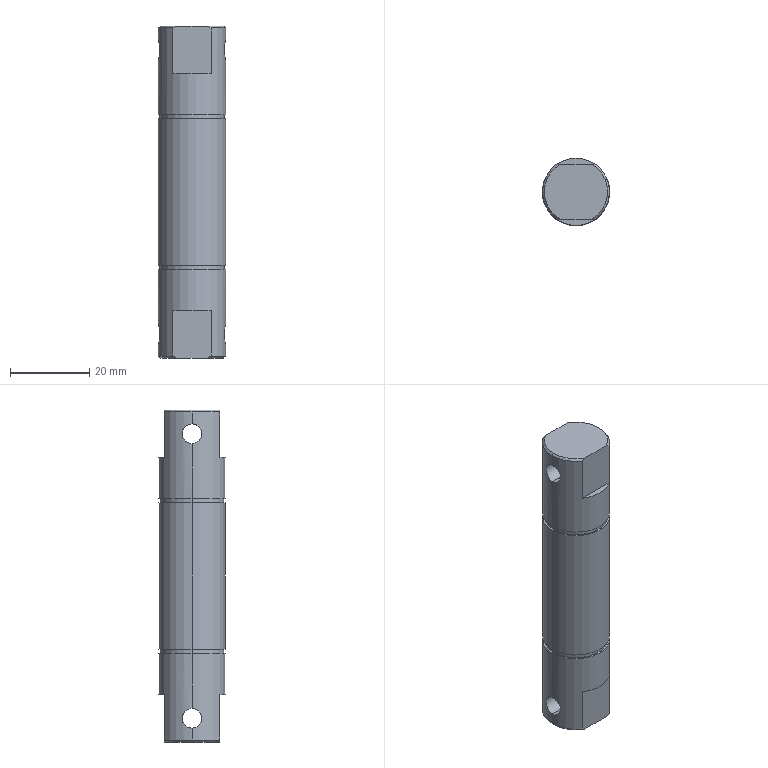Part | SolidWorks | features Chamfer 1, Extrusion 1, HoleWzd 1, ICE 1, MirrorPattern 1, RevCut 1 | 1 solid | 34 faces | box 17 x 17 x 84 mm | volume 17880 mm3 | cylinder 14 | plane 14 | cone 6 | commonest cylinder face diameters 17 x6 5 x4 16.2 x4
STEP:
#1=CARTESIAN_POINT('',(4.822,7.,41.5));
#2=VERTEX_POINT('',#1);
#3=CARTESIAN_POINT('',(8.5,0.,41.5));
#4=VERTEX_POINT('',#3);
#5=CARTESIAN_POINT('',(0.,0.,41.5));
#6=DIRECTION('',(0.,0.,-1.));
#7=DIRECTION('',(1.,0.,0.));
#8=AXIS2_PLACEMENT_3D('',#5,#6,#7);
#9=CIRCLE('',#8,8.5);
#10=EDGE_CURVE('',#2,#4,#9,.T.);
#11=ORIENTED_EDGE('',*,*,#10,.T.);
#12=CARTESIAN_POINT('',(8.5,0.,38.5));
#13=VERTEX_POINT('',#12);
#14=CARTESIAN_POINT('',(8.5,0.,42.));
#15=DIRECTION('',(0.,0.,-1.));
#16=VECTOR('',#15,1000.);
#17=LINE('',#14,#16);
#18=EDGE_CURVE('',#4,#13,#17,.T.);
#19=ORIENTED_EDGE('',*,*,#18,.T.);
#20=CARTESIAN_POINT('',(8.5,0.,33.5));
#21=VERTEX_POINT('',#20);
#22=CARTESIAN_POINT('',(8.5,0.,38.5));
#23=CARTESIAN_POINT('',(8.5,0.3274,38.5));
#24=CARTESIAN_POINT('',(8.48,0.658,38.434));
#25=CARTESIAN_POINT('',(8.429,1.11,38.246));
#26=CARTESIAN_POINT('',(8.408,1.256,38.168));
#27=CARTESIAN_POINT('',(8.363,1.527,37.986));
#28=CARTESIAN_POINT('',(8.339,1.652,37.883));
#29=CARTESIAN_POINT('',(8.29,1.883,37.653));
#30=CARTESIAN_POINT('',(8.265,1.987,37.525));
#31=CARTESIAN_POINT('',(8.219,2.168,37.256));
#32=CARTESIAN_POINT('',(8.198,2.245,37.113));
#33=CARTESIAN_POINT('',(8.163,2.372,36.808));
#34=CARTESIAN_POINT('',(8.149,2.419,36.651));
#35=CARTESIAN_POINT('',(8.129,2.483,36.331));
#36=CARTESIAN_POINT('',(8.124,2.5,36.165));
#37=CARTESIAN_POINT('',(8.124,2.5,35.835));
#38=CARTESIAN_POINT('',(8.129,2.484,35.673));
#39=CARTESIAN_POINT('',(8.148,2.42,35.351));
#40=CARTESIAN_POINT('',(8.163,2.371,35.191));
#41=CARTESIAN_POINT('',(8.216,2.183,34.739));
#42=CARTESIAN_POINT('',(8.265,1.998,34.462));
#43=CARTESIAN_POINT('',(8.338,1.654,34.118));
#44=CARTESIAN_POINT('',(8.363,1.527,34.013));
#45=CARTESIAN_POINT('',(8.408,1.255,33.832));
#46=CARTESIAN_POINT('',(8.428,1.112,33.755));
#47=CARTESIAN_POINT('',(8.463,0.8109,33.63));
#48=CARTESIAN_POINT('',(8.477,0.6512,33.581));
#49=CARTESIAN_POINT('',(8.495,0.3296,33.516));
#50=CARTESIAN_POINT('',(8.5,0.1661,33.5));
#51=CARTESIAN_POINT('',(8.5,0.,33.5));
#52=B_SPLINE_CURVE_WITH_KNOTS('',3,(#22,#23,#24,#25,#26,#27,#28,#29,#30,#31,#32,#33,#34,#35,#36,#37,#38,#39,#40,#41,#42,#43,#44,#45,#46,#47,#48,#49,#50,#51),.UNSPECIFIED.,.F.,.F.,(4,2,2,2,2,2,2,2,2,2,2,2,2,2,4),(0.00786,0.008842,0.009333,0.009824,0.01032,0.01081,0.0113,0.01179,0.01228,0.01277,0.01375,0.01424,0.01474,0.01523,0.01572),.UNSPECIFIED.);
#53=EDGE_CURVE('',#13,#21,#52,.T.);
#54=ORIENTED_EDGE('',*,*,#53,.T.);
#55=CARTESIAN_POINT('',(8.5,0.,19.6));
#56=VERTEX_POINT('',#55);
#57=CARTESIAN_POINT('',(8.5,0.,42.));
#58=DIRECTION('',(0.,0.,-1.));
#59=VECTOR('',#58,1000.);
#60=LINE('',#57,#59);
#61=EDGE_CURVE('',#21,#56,#60,.T.);
#62=ORIENTED_EDGE('',*,*,#61,.T.);
#63=CARTESIAN_POINT('',(-8.5,0.,19.6));
#64=VERTEX_POINT('',#63);
#65=CARTESIAN_POINT('',(0.,0.,19.6));
#66=DIRECTION('',(0.,0.,1.));
#67=DIRECTION('',(1.,0.,0.));
#68=AXIS2_PLACEMENT_3D('',#65,#66,#67);
#69=CIRCLE('',#68,8.5);
#70=EDGE_CURVE('',#56,#64,#69,.T.);
#71=ORIENTED_EDGE('',*,*,#70,.T.);
#72=CARTESIAN_POINT('',(-8.5,0.,33.5));
#73=VERTEX_POINT('',#72);
#74=CARTESIAN_POINT('',(-8.5,0.,42.));
#75=DIRECTION('',(0.,0.,-1.));
#76=VECTOR('',#75,1000.);
#77=LINE('',#74,#76);
#78=EDGE_CURVE('',#73,#64,#77,.T.);
#79=ORIENTED_EDGE('',*,*,#78,.F.);
#80=CARTESIAN_POINT('',(-8.5,0.,38.5));
#81=VERTEX_POINT('',#80);
#82=CARTESIAN_POINT('',(-8.5,0.,33.5));
#83=CARTESIAN_POINT('',(-8.5,0.1662,33.5));
#84=CARTESIAN_POINT('',(-8.495,0.3294,33.516));
#85=CARTESIAN_POINT('',(-8.477,0.6502,33.58));
#86=CARTESIAN_POINT('',(-8.463,0.8095,33.629));
#87=CARTESIAN_POINT('',(-8.428,1.112,33.755));
#88=CARTESIAN_POINT('',(-8.408,1.255,33.832));
#89=CARTESIAN_POINT('',(-8.363,1.526,34.013));
#90=CARTESIAN_POINT('',(-8.338,1.654,34.118));
#91=CARTESIAN_POINT('',(-8.265,1.998,34.462));
#92=CARTESIAN_POINT('',(-8.216,2.183,34.74));
#93=CARTESIAN_POINT('',(-8.163,2.371,35.19));
#94=CARTESIAN_POINT('',(-8.149,2.419,35.349));
#95=CARTESIAN_POINT('',(-8.129,2.484,35.672));
#96=CARTESIAN_POINT('',(-8.124,2.5,35.835));
#97=CARTESIAN_POINT('',(-8.124,2.5,36.163));
#98=CARTESIAN_POINT('',(-8.129,2.484,36.33));
#99=CARTESIAN_POINT('',(-8.149,2.419,36.651));
#100=CARTESIAN_POINT('',(-8.163,2.372,36.807));
#101=CARTESIAN_POINT('',(-8.216,2.182,37.263));
#102=CARTESIAN_POINT('',(-8.265,1.998,37.538));
#103=CARTESIAN_POINT('',(-8.339,1.652,37.884));
#104=CARTESIAN_POINT('',(-8.363,1.526,37.987));
#105=CARTESIAN_POINT('',(-8.408,1.256,38.168));
#106=CARTESIAN_POINT('',(-8.429,1.11,38.246));
#107=CARTESIAN_POINT('',(-8.463,0.8084,38.371));
#108=CARTESIAN_POINT('',(-8.476,0.6525,38.419));
#109=CARTESIAN_POINT('',(-8.495,0.3297,38.484));
#110=CARTESIAN_POINT('',(-8.5,0.1637,38.5));
#111=CARTESIAN_POINT('',(-8.5,0.,38.5));
#112=B_SPLINE_CURVE_WITH_KNOTS('',3,(#82,#83,#84,#85,#86,#87,#88,#89,#90,#91,#92,#93,#94,#95,#96,#97,#98,#99,#100,#101,#102,#103,#104,#105,#106,#107,#108,#109,#110,#111),.UNSPECIFIED.,.F.,.F.,(4,2,2,2,2,2,2,2,2,2,2,2,2,2,4),(0.,0.0004912,0.0009825,0.001474,0.001965,0.002947,0.003439,0.00393,0.004421,0.004912,0.005895,0.006386,0.006877,0.007369,0.00786),.UNSPECIFIED.);
#113=EDGE_CURVE('',#73,#81,#112,.T.);
#114=ORIENTED_EDGE('',*,*,#113,.T.);
#115=CARTESIAN_POINT('',(-8.5,0.,41.5));
#116=VERTEX_POINT('',#115);
#117=CARTESIAN_POINT('',(-8.5,0.,42.));
#118=DIRECTION('',(0.,0.,-1.));
#119=VECTOR('',#118,1000.);
#120=LINE('',#117,#119);
#121=EDGE_CURVE('',#116,#81,#120,.T.);
#122=ORIENTED_EDGE('',*,*,#121,.F.);
#123=CARTESIAN_POINT('',(-4.822,7.,41.5));
#124=VERTEX_POINT('',#123);
#125=CARTESIAN_POINT('',(0.,0.,41.5));
#126=DIRECTION('',(0.,0.,-1.));
#127=DIRECTION('',(1.,0.,0.));
#128=AXIS2_PLACEMENT_3D('',#125,#126,#127);
#129=CIRCLE('',#128,8.5);
#130=EDGE_CURVE('',#116,#124,#129,.T.);
#131=ORIENTED_EDGE('',*,*,#130,.T.);
#132=CARTESIAN_POINT('',(-4.822,7.,30.));
#133=VERTEX_POINT('',#132);
#134=CARTESIAN_POINT('',(-4.822,7.,42.));
#135=DIRECTION('',(0.,0.,-1.));
#136=VECTOR('',#135,1000.);
#137=LINE('',#134,#136);
#138=EDGE_CURVE('',#124,#133,#137,.T.);
#139=ORIENTED_EDGE('',*,*,#138,.T.);
#140=CARTESIAN_POINT('',(4.822,7.,30.));
#141=VERTEX_POINT('',#140);
#142=CARTESIAN_POINT('',(0.,0.,30.));
#143=DIRECTION('',(0.,0.,1.));
#144=DIRECTION('',(1.,0.,0.));
#145=AXIS2_PLACEMENT_3D('',#142,#143,#144);
#146=CIRCLE('',#145,8.5);
#147=EDGE_CURVE('',#141,#133,#146,.T.);
#148=ORIENTED_EDGE('',*,*,#147,.F.);
#149=CARTESIAN_POINT('',(4.822,7.,42.));
#150=DIRECTION('',(0.,0.,1.));
#151=VECTOR('',#150,1000.);
#152=LINE('',#149,#151);
#153=EDGE_CURVE('',#141,#2,#152,.T.);
#154=ORIENTED_EDGE('',*,*,#153,.T.);
#155=EDGE_LOOP('',(#11,#19,#54,#62,#71,#79,#114,#122,#131,#139,#148,#154));
#156=FACE_OUTER_BOUND('',#155,.T.);
#157=CARTESIAN_POINT('',(0.,0.,42.));
#158=DIRECTION('',(0.,0.,-1.));
#159=DIRECTION('',(-1.,0.,0.));
#160=AXIS2_PLACEMENT_3D('',#157,#158,#159);
#161=CYLINDRICAL_SURFACE('',#160,8.5);
#162=ADVANCED_FACE('',(#156),#161,.T.);
#163=CARTESIAN_POINT('',(-8.,0.,42.));
#164=VERTEX_POINT('',#163);
#165=CARTESIAN_POINT('',(-3.873,-7.,42.));
#166=VERTEX_POINT('',#165);
#167=CARTESIAN_POINT('',(0.,0.,42.));
#168=DIRECTION('',(0.,0.,1.));
#169=DIRECTION('',(1.,0.,0.));
#170=AXIS2_PLACEMENT_3D('',#167,#168,#169);
#171=CIRCLE('',#170,8.);
#172=EDGE_CURVE('',#164,#166,#171,.T.);
#173=ORIENTED_EDGE('',*,*,#172,.F.);
#174=CARTESIAN_POINT('',(-8.,0.,42.));
#175=DIRECTION('',(-0.7071,0.,-0.7071));
#176=VECTOR('',#175,1000.);
#177=LINE('',#174,#176);
#178=EDGE_CURVE('',#164,#116,#177,.T.);
#179=ORIENTED_EDGE('',*,*,#178,.T.);
#180=CARTESIAN_POINT('',(-4.822,-7.,41.5));
#181=VERTEX_POINT('',#180);
#182=CARTESIAN_POINT('',(0.,0.,41.5));
#183=DIRECTION('',(0.,0.,-1.));
#184=DIRECTION('',(1.,0.,0.));
#185=AXIS2_PLACEMENT_3D('',#182,#183,#184);
#186=CIRCLE('',#185,8.5);
#187=EDGE_CURVE('',#181,#116,#186,.T.);
#188=ORIENTED_EDGE('',*,*,#187,.F.);
#189=CARTESIAN_POINT('',(-3.873,-7.,42.));
#190=CARTESIAN_POINT('',(-4.195,-7.,41.844));
#191=CARTESIAN_POINT('',(-4.511,-7.,41.676));
#192=CARTESIAN_POINT('',(-4.822,-7.,41.5));
#193=B_SPLINE_CURVE_WITH_KNOTS('',3,(#189,#190,#191,#192),.UNSPECIFIED.,.F.,.F.,(4,4),(0.,0.001073),.UNSPECIFIED.);
#194=EDGE_CURVE('',#166,#181,#193,.T.);
#195=ORIENTED_EDGE('',*,*,#194,.F.);
#196=EDGE_LOOP('',(#173,#179,#188,#195));
#197=FACE_OUTER_BOUND('',#196,.T.);
#198=CARTESIAN_POINT('',(0.,0.,42.));
#199=DIRECTION('',(0.,0.,-1.));
#200=DIRECTION('',(-1.,0.,0.));
#201=AXIS2_PLACEMENT_3D('',#198,#199,#200);
#202=CONICAL_SURFACE('',#201,8.,0.7854);
#203=ADVANCED_FACE('',(#197),#202,.T.);
#204=CARTESIAN_POINT('',(-8.5,0.,38.5));
#205=CARTESIAN_POINT('',(-8.5,-0.3274,38.5));
#206=CARTESIAN_POINT('',(-8.48,-0.658,38.434));
#207=CARTESIAN_POINT('',(-8.429,-1.11,38.246));
#208=CARTESIAN_POINT('',(-8.408,-1.256,38.168));
#209=CARTESIAN_POINT('',(-8.363,-1.527,37.986));
#210=CARTESIAN_POINT('',(-8.339,-1.652,37.883));
#211=CARTESIAN_POINT('',(-8.29,-1.883,37.653));
#212=CARTESIAN_POINT('',(-8.265,-1.987,37.525));
#213=CARTESIAN_POINT('',(-8.219,-2.168,37.256));
#214=CARTESIAN_POINT('',(-8.198,-2.245,37.113));
#215=CARTESIAN_POINT('',(-8.163,-2.372,36.808));
#216=CARTESIAN_POINT('',(-8.149,-2.419,36.651));
#217=CARTESIAN_POINT('',(-8.129,-2.483,36.331));
#218=CARTESIAN_POINT('',(-8.124,-2.5,36.165));
#219=CARTESIAN_POINT('',(-8.124,-2.5,35.835));
#220=CARTESIAN_POINT('',(-8.129,-2.484,35.673));
#221=CARTESIAN_POINT('',(-8.148,-2.42,35.351));
#222=CARTESIAN_POINT('',(-8.163,-2.371,35.191));
#223=CARTESIAN_POINT('',(-8.216,-2.183,34.739));
#224=CARTESIAN_POINT('',(-8.265,-1.998,34.462));
#225=CARTESIAN_POINT('',(-8.338,-1.654,34.118));
#226=CARTESIAN_POINT('',(-8.363,-1.527,34.013));
#227=CARTESIAN_POINT('',(-8.408,-1.255,33.832));
#228=CARTESIAN_POINT('',(-8.428,-1.112,33.755));
#229=CARTESIAN_POINT('',(-8.463,-0.8109,33.63));
#230=CARTESIAN_POINT('',(-8.477,-0.6512,33.581));
#231=CARTESIAN_POINT('',(-8.495,-0.3296,33.516));
#232=CARTESIAN_POINT('',(-8.5,-0.1661,33.5));
#233=CARTESIAN_POINT('',(-8.5,0.,33.5));
#234=B_SPLINE_CURVE_WITH_KNOTS('',3,(#204,#205,#206,#207,#208,#209,#210,#211,#212,#213,#214,#215,#216,#217,#218,#219,#220,#221,#222,#223,#224,#225,#226,#227,#228,#229,#230,#231,#232,#233),.UNSPECIFIED.,.F.,.F.,(4,2,2,2,2,2,2,2,2,2,2,2,2,2,4),(0.00786,0.008842,0.009333,0.009824,0.01032,0.01081,0.0113,0.01179,0.01228,0.01277,0.01375,0.01424,0.01474,0.01523,0.01572),.UNSPECIFIED.);
#235=EDGE_CURVE('',#81,#73,#234,.T.);
#236=ORIENTED_EDGE('',*,*,#235,.F.);
#237=CARTESIAN_POINT('',(8.5,0.,38.5));
#238=DIRECTION('',(1.,0.,0.));
#239=VECTOR('',#238,1000.);
#240=LINE('',#237,#239);
#241=EDGE_CURVE('',#81,#13,#240,.T.);
#242=ORIENTED_EDGE('',*,*,#241,.T.);
#243=CARTESIAN_POINT('',(8.5,0.,33.5));
#244=CARTESIAN_POINT('',(8.5,-0.1662,33.5));
#245=CARTESIAN_POINT('',(8.495,-0.3294,33.516));
#246=CARTESIAN_POINT('',(8.477,-0.6502,33.58));
#247=CARTESIAN_POINT('',(8.463,-0.8095,33.629));
#248=CARTESIAN_POINT('',(8.428,-1.112,33.755));
#249=CARTESIAN_POINT('',(8.408,-1.255,33.832));
#250=CARTESIAN_POINT('',(8.363,-1.526,34.013));
#251=CARTESIAN_POINT('',(8.338,-1.654,34.118));
#252=CARTESIAN_POINT('',(8.265,-1.998,34.462));
#253=CARTESIAN_POINT('',(8.216,-2.183,34.74));
#254=CARTESIAN_POINT('',(8.163,-2.371,35.19));
#255=CARTESIAN_POINT('',(8.149,-2.419,35.349));
#256=CARTESIAN_POINT('',(8.129,-2.484,35.672));
#257=CARTESIAN_POINT('',(8.124,-2.5,35.835));
#258=CARTESIAN_POINT('',(8.124,-2.5,36.163));
#259=CARTESIAN_POINT('',(8.129,-2.484,36.33));
#260=CARTESIAN_POINT('',(8.149,-2.419,36.651));
#261=CARTESIAN_POINT('',(8.163,-2.372,36.807));
#262=CARTESIAN_POINT('',(8.216,-2.182,37.263));
#263=CARTESIAN_POINT('',(8.265,-1.998,37.538));
#264=CARTESIAN_POINT('',(8.339,-1.652,37.884));
#265=CARTESIAN_POINT('',(8.363,-1.526,37.987));
#266=CARTESIAN_POINT('',(8.408,-1.256,38.168));
#267=CARTESIAN_POINT('',(8.429,-1.11,38.246));
#268=CARTESIAN_POINT('',(8.463,-0.8084,38.371));
#269=CARTESIAN_POINT('',(8.476,-0.6525,38.419));
#270=CARTESIAN_POINT('',(8.495,-0.3297,38.484));
#271=CARTESIAN_POINT('',(8.5,-0.1637,38.5));
#272=CARTESIAN_POINT('',(8.5,0.,38.5));
#273=B_SPLINE_CURVE_WITH_KNOTS('',3,(#243,#244,#245,#246,#247,#248,#249,#250,#251,#252,#253,#254,#255,#256,#257,#258,#259,#260,#261,#262,#263,#264,#265,#266,#267,#268,#269,#270,#271,#272),.UNSPECIFIED.,.F.,.F.,(4,2,2,2,2,2,2,2,2,2,2,2,2,2,4),(0.,0.0004912,0.0009825,0.001474,0.001965,0.002947,0.003439,0.00393,0.004421,0.004912,0.005895,0.006386,0.006877,0.007369,0.00786),.UNSPECIFIED.);
#274=EDGE_CURVE('',#21,#13,#273,.T.);
#275=ORIENTED_EDGE('',*,*,#274,.F.);
#276=CARTESIAN_POINT('',(8.5,0.,33.5));
#277=DIRECTION('',(1.,0.,0.));
#278=VECTOR('',#277,1000.);
#279=LINE('',#276,#278);
#280=EDGE_CURVE('',#73,#21,#279,.T.);
#281=ORIENTED_EDGE('',*,*,#280,.F.);
#282=EDGE_LOOP('',(#236,#242,#275,#281));
#283=FACE_OUTER_BOUND('',#282,.T.);
#284=CARTESIAN_POINT('',(8.5,0.,36.));
#285=DIRECTION('',(1.,0.,0.));
#286=DIRECTION('',(0.,0.,-1.));
#287=AXIS2_PLACEMENT_3D('',#284,#285,#286);
#288=CYLINDRICAL_SURFACE('',#287,2.5);
#289=ADVANCED_FACE('',(#283),#288,.F.);
#290=CARTESIAN_POINT('',(8.1,0.,18.5));
#291=VERTEX_POINT('',#290);
#292=CARTESIAN_POINT('',(-8.1,0.,18.5));
#293=VERTEX_POINT('',#292);
#294=CARTESIAN_POINT('',(0.,0.,18.5));
#295=DIRECTION('',(0.,0.,1.));
#296=DIRECTION('',(1.,0.,0.));
#297=AXIS2_PLACEMENT_3D('',#294,#295,#296);
#298=CIRCLE('',#297,8.1);
#299=EDGE_CURVE('',#291,#293,#298,.T.);
#300=ORIENTED_EDGE('',*,*,#299,.T.);
#301=CARTESIAN_POINT('',(-8.1,0.,19.6));
#302=VERTEX_POINT('',#301);
#303=CARTESIAN_POINT('',(-8.1,0.,0.));
#304=DIRECTION('',(0.,0.,1.));
#305=VECTOR('',#304,1000.);
#306=LINE('',#303,#305);
#307=EDGE_CURVE('',#293,#302,#306,.T.);
#308=ORIENTED_EDGE('',*,*,#307,.T.);
#309=CARTESIAN_POINT('',(8.1,0.,19.6));
#310=VERTEX_POINT('',#309);
#311=CARTESIAN_POINT('',(0.,0.,19.6));
#312=DIRECTION('',(0.,0.,1.));
#313=DIRECTION('',(1.,0.,0.));
#314=AXIS2_PLACEMENT_3D('',#311,#312,#313);
#315=CIRCLE('',#314,8.1);
#316=EDGE_CURVE('',#310,#302,#315,.T.);
#317=ORIENTED_EDGE('',*,*,#316,.F.);
#318=CARTESIAN_POINT('',(8.1,0.,0.));
#319=DIRECTION('',(0.,0.,1.));
#320=VECTOR('',#319,1000.);
#321=LINE('',#318,#320);
#322=EDGE_CURVE('',#291,#310,#321,.T.);
#323=ORIENTED_EDGE('',*,*,#322,.F.);
#324=EDGE_LOOP('',(#300,#308,#317,#323));
#325=FACE_OUTER_BOUND('',#324,.T.);
#326=CARTESIAN_POINT('',(0.,0.,0.));
#327=DIRECTION('',(0.,0.,1.));
#328=DIRECTION('',(1.,0.,0.));
#329=AXIS2_PLACEMENT_3D('',#326,#327,#328);
#330=CYLINDRICAL_SURFACE('',#329,8.1);
#331=ADVANCED_FACE('',(#325),#330,.T.);
#332=CARTESIAN_POINT('',(8.5,0.,18.5));
#333=VERTEX_POINT('',#332);
#334=CARTESIAN_POINT('',(-8.5,0.,18.5));
#335=VERTEX_POINT('',#334);
#336=CARTESIAN_POINT('',(0.,0.,18.5));
#337=DIRECTION('',(0.,0.,1.));
#338=DIRECTION('',(1.,0.,0.));
#339=AXIS2_PLACEMENT_3D('',#336,#337,#338);
#340=CIRCLE('',#339,8.5);
#341=EDGE_CURVE('',#333,#335,#340,.T.);
#342=ORIENTED_EDGE('',*,*,#341,.F.);
#343=CARTESIAN_POINT('',(8.5,0.,-18.5));
#344=VERTEX_POINT('',#343);
#345=CARTESIAN_POINT('',(8.5,0.,42.));
#346=DIRECTION('',(0.,0.,-1.));
#347=VECTOR('',#346,1000.);
#348=LINE('',#345,#347);
#349=EDGE_CURVE('',#333,#344,#348,.T.);
#350=ORIENTED_EDGE('',*,*,#349,.T.);
#351=CARTESIAN_POINT('',(-8.5,0.,-18.5));
#352=VERTEX_POINT('',#351);
#353=CARTESIAN_POINT('',(0.,0.,-18.5));
#354=DIRECTION('',(0.,0.,1.));
#355=DIRECTION('',(1.,0.,0.));
#356=AXIS2_PLACEMENT_3D('',#353,#354,#355);
#357=CIRCLE('',#356,8.5);
#358=EDGE_CURVE('',#344,#352,#357,.T.);
#359=ORIENTED_EDGE('',*,*,#358,.T.);
#360=CARTESIAN_POINT('',(-8.5,0.,42.));
#361=DIRECTION('',(0.,0.,-1.));
#362=VECTOR('',#361,1000.);
#363=LINE('',#360,#362);
#364=EDGE_CURVE('',#335,#352,#363,.T.);
#365=ORIENTED_EDGE('',*,*,#364,.F.);
#366=EDGE_LOOP('',(#342,#350,#359,#365));
#367=FACE_OUTER_BOUND('',#366,.T.);
#368=CARTESIAN_POINT('',(0.,0.,42.));
#369=DIRECTION('',(0.,0.,-1.));
#370=DIRECTION('',(-1.,0.,0.));
#371=AXIS2_PLACEMENT_3D('',#368,#369,#370);
#372=CYLINDRICAL_SURFACE('',#371,8.5);
#373=ADVANCED_FACE('',(#367),#372,.T.);
#374=CARTESIAN_POINT('',(8.1,0.,-19.6));
#375=VERTEX_POINT('',#374);
#376=CARTESIAN_POINT('',(-8.1,0.,-19.6));
#377=VERTEX_POINT('',#376);
#378=CARTESIAN_POINT('',(0.,0.,-19.6));
#379=DIRECTION('',(0.,0.,1.));
#380=DIRECTION('',(1.,0.,0.));
#381=AXIS2_PLACEMENT_3D('',#378,#379,#380);
#382=CIRCLE('',#381,8.1);
#383=EDGE_CURVE('',#375,#377,#382,.T.);
#384=ORIENTED_EDGE('',*,*,#383,.T.);
#385=CARTESIAN_POINT('',(-8.1,0.,-18.5));
#386=VERTEX_POINT('',#385);
#387=CARTESIAN_POINT('',(-8.1,0.,0.));
#388=DIRECTION('',(0.,0.,1.));
#389=VECTOR('',#388,1000.);
#390=LINE('',#387,#389);
#391=EDGE_CURVE('',#377,#386,#390,.T.);
#392=ORIENTED_EDGE('',*,*,#391,.T.);
#393=CARTESIAN_POINT('',(8.1,0.,-18.5));
#394=VERTEX_POINT('',#393);
#395=CARTESIAN_POINT('',(0.,0.,-18.5));
#396=DIRECTION('',(0.,0.,1.));
#397=DIRECTION('',(1.,0.,0.));
#398=AXIS2_PLACEMENT_3D('',#395,#396,#397);
#399=CIRCLE('',#398,8.1);
#400=EDGE_CURVE('',#394,#386,#399,.T.);
#401=ORIENTED_EDGE('',*,*,#400,.F.);
#402=CARTESIAN_POINT('',(8.1,0.,0.));
#403=DIRECTION('',(0.,0.,1.));
#404=VECTOR('',#403,1000.);
#405=LINE('',#402,#404);
#406=EDGE_CURVE('',#375,#394,#405,.T.);
#407=ORIENTED_EDGE('',*,*,#406,.F.);
#408=EDGE_LOOP('',(#384,#392,#401,#407));
#409=FACE_OUTER_BOUND('',#408,.T.);
#410=CARTESIAN_POINT('',(0.,0.,0.));
#411=DIRECTION('',(0.,0.,1.));
#412=DIRECTION('',(1.,0.,0.));
#413=AXIS2_PLACEMENT_3D('',#410,#411,#412);
#414=CYLINDRICAL_SURFACE('',#413,8.1);
#415=ADVANCED_FACE('',(#409),#414,.T.);
#416=CARTESIAN_POINT('',(-8.5,0.,-33.5));
#417=VERTEX_POINT('',#416);
#418=CARTESIAN_POINT('',(-8.5,0.,-38.5));
#419=VERTEX_POINT('',#418);
#420=CARTESIAN_POINT('',(-8.5,0.,-33.5));
#421=CARTESIAN_POINT('',(-8.5,-0.3274,-33.5));
#422=CARTESIAN_POINT('',(-8.48,-0.658,-33.566));
#423=CARTESIAN_POINT('',(-8.429,-1.11,-33.754));
#424=CARTESIAN_POINT('',(-8.408,-1.256,-33.832));
#425=CARTESIAN_POINT('',(-8.363,-1.527,-34.014));
#426=CARTESIAN_POINT('',(-8.339,-1.652,-34.117));
#427=CARTESIAN_POINT('',(-8.29,-1.883,-34.347));
#428=CARTESIAN_POINT('',(-8.265,-1.987,-34.475));
#429=CARTESIAN_POINT('',(-8.219,-2.168,-34.744));
#430=CARTESIAN_POINT('',(-8.198,-2.245,-34.887));
#431=CARTESIAN_POINT('',(-8.163,-2.372,-35.192));
#432=CARTESIAN_POINT('',(-8.149,-2.419,-35.349));
#433=CARTESIAN_POINT('',(-8.129,-2.483,-35.669));
#434=CARTESIAN_POINT('',(-8.124,-2.5,-35.835));
#435=CARTESIAN_POINT('',(-8.124,-2.5,-36.165));
#436=CARTESIAN_POINT('',(-8.129,-2.484,-36.327));
#437=CARTESIAN_POINT('',(-8.148,-2.42,-36.649));
#438=CARTESIAN_POINT('',(-8.163,-2.371,-36.809));
#439=CARTESIAN_POINT('',(-8.216,-2.183,-37.261));
#440=CARTESIAN_POINT('',(-8.265,-1.998,-37.538));
#441=CARTESIAN_POINT('',(-8.338,-1.654,-37.882));
#442=CARTESIAN_POINT('',(-8.363,-1.527,-37.987));
#443=CARTESIAN_POINT('',(-8.408,-1.255,-38.168));
#444=CARTESIAN_POINT('',(-8.428,-1.112,-38.245));
#445=CARTESIAN_POINT('',(-8.463,-0.8109,-38.37));
#446=CARTESIAN_POINT('',(-8.477,-0.6512,-38.419));
#447=CARTESIAN_POINT('',(-8.495,-0.3296,-38.484));
#448=CARTESIAN_POINT('',(-8.5,-0.1661,-38.5));
#449=CARTESIAN_POINT('',(-8.5,0.,-38.5));
#450=B_SPLINE_CURVE_WITH_KNOTS('',3,(#420,#421,#422,#423,#424,#425,#426,#427,#428,#429,#430,#431,#432,#433,#434,#435,#436,#437,#438,#439,#440,#441,#442,#443,#444,#445,#446,#447,#448,#449),.UNSPECIFIED.,.F.,.F.,(4,2,2,2,2,2,2,2,2,2,2,2,2,2,4),(0.00786,0.008842,0.009333,0.009824,0.01032,0.01081,0.0113,0.01179,0.01228,0.01277,0.01375,0.01424,0.01474,0.01523,0.01572),.UNSPECIFIED.);
#451=EDGE_CURVE('',#417,#419,#450,.T.);
#452=ORIENTED_EDGE('',*,*,#451,.F.);
#453=CARTESIAN_POINT('',(8.5,0.,-33.5));
#454=VERTEX_POINT('',#453);
#455=CARTESIAN_POINT('',(8.5,0.,-33.5));
#456=DIRECTION('',(1.,0.,0.));
#457=VECTOR('',#456,1000.);
#458=LINE('',#455,#457);
#459=EDGE_CURVE('',#417,#454,#458,.T.);
#460=ORIENTED_EDGE('',*,*,#459,.T.);
#461=CARTESIAN_POINT('',(8.5,0.,-38.5));
#462=VERTEX_POINT('',#461);
#463=CARTESIAN_POINT('',(8.5,0.,-38.5));
#464=CARTESIAN_POINT('',(8.5,-0.1662,-38.5));
#465=CARTESIAN_POINT('',(8.495,-0.3294,-38.484));
#466=CARTESIAN_POINT('',(8.477,-0.6502,-38.42));
#467=CARTESIAN_POINT('',(8.463,-0.8095,-38.371));
#468=CARTESIAN_POINT('',(8.428,-1.112,-38.245));
#469=CARTESIAN_POINT('',(8.408,-1.255,-38.168));
#470=CARTESIAN_POINT('',(8.363,-1.526,-37.987));
#471=CARTESIAN_POINT('',(8.338,-1.654,-37.882));
#472=CARTESIAN_POINT('',(8.265,-1.998,-37.538));
#473=CARTESIAN_POINT('',(8.216,-2.183,-37.26));
#474=CARTESIAN_POINT('',(8.163,-2.371,-36.81));
#475=CARTESIAN_POINT('',(8.149,-2.419,-36.651));
#476=CARTESIAN_POINT('',(8.129,-2.484,-36.328));
#477=CARTESIAN_POINT('',(8.124,-2.5,-36.165));
#478=CARTESIAN_POINT('',(8.124,-2.5,-35.837));
#479=CARTESIAN_POINT('',(8.129,-2.484,-35.67));
#480=CARTESIAN_POINT('',(8.149,-2.419,-35.349));
#481=CARTESIAN_POINT('',(8.163,-2.372,-35.193));
#482=CARTESIAN_POINT('',(8.216,-2.182,-34.737));
#483=CARTESIAN_POINT('',(8.265,-1.998,-34.462));
#484=CARTESIAN_POINT('',(8.339,-1.652,-34.116));
#485=CARTESIAN_POINT('',(8.363,-1.526,-34.013));
#486=CARTESIAN_POINT('',(8.408,-1.256,-33.832));
#487=CARTESIAN_POINT('',(8.429,-1.11,-33.754));
#488=CARTESIAN_POINT('',(8.463,-0.8084,-33.629));
#489=CARTESIAN_POINT('',(8.476,-0.6525,-33.581));
#490=CARTESIAN_POINT('',(8.495,-0.3297,-33.516));
#491=CARTESIAN_POINT('',(8.5,-0.1637,-33.5));
#492=CARTESIAN_POINT('',(8.5,0.,-33.5));
#493=B_SPLINE_CURVE_WITH_KNOTS('',3,(#463,#464,#465,#466,#467,#468,#469,#470,#471,#472,#473,#474,#475,#476,#477,#478,#479,#480,#481,#482,#483,#484,#485,#486,#487,#488,#489,#490,#491,#492),.UNSPECIFIED.,.F.,.F.,(4,2,2,2,2,2,2,2,2,2,2,2,2,2,4),(0.,0.0004912,0.0009825,0.001474,0.001965,0.002947,0.003439,0.00393,0.004421,0.004912,0.005895,0.006386,0.006877,0.007369,0.00786),.UNSPECIFIED.);
#494=EDGE_CURVE('',#462,#454,#493,.T.);
#495=ORIENTED_EDGE('',*,*,#494,.F.);
#496=CARTESIAN_POINT('',(8.5,0.,-38.5));
#497=DIRECTION('',(1.,0.,0.));
#498=VECTOR('',#497,1000.);
#499=LINE('',#496,#498);
#500=EDGE_CURVE('',#419,#462,#499,.T.);
#501=ORIENTED_EDGE('',*,*,#500,.F.);
#502=EDGE_LOOP('',(#452,#460,#495,#501));
#503=FACE_OUTER_BOUND('',#502,.T.);
#504=CARTESIAN_POINT('',(8.5,0.,-36.));
#505=DIRECTION('',(1.,0.,0.));
#506=DIRECTION('',(0.,0.,-1.));
#507=AXIS2_PLACEMENT_3D('',#504,#505,#506);
#508=CYLINDRICAL_SURFACE('',#507,2.5);
#509=ADVANCED_FACE('',(#503),#508,.F.);
#510=CARTESIAN_POINT('',(8.,0.,-42.));
#511=VERTEX_POINT('',#510);
#512=CARTESIAN_POINT('',(3.873,-7.,-42.));
#513=VERTEX_POINT('',#512);
#514=CARTESIAN_POINT('',(0.,0.,-42.));
#515=DIRECTION('',(0.,0.,-1.));
#516=DIRECTION('',(1.,0.,0.));
#517=AXIS2_PLACEMENT_3D('',#514,#515,#516);
#518=CIRCLE('',#517,8.);
#519=EDGE_CURVE('',#511,#513,#518,.T.);
#520=ORIENTED_EDGE('',*,*,#519,.F.);
#521=CARTESIAN_POINT('',(8.5,0.,-41.5));
#522=VERTEX_POINT('',#521);
#523=CARTESIAN_POINT('',(8.5,0.,-41.5));
#524=DIRECTION('',(0.7071,0.,0.7071));
#525=VECTOR('',#524,1000.);
#526=LINE('',#523,#525);
#527=EDGE_CURVE('',#511,#522,#526,.T.);
#528=ORIENTED_EDGE('',*,*,#527,.T.);
#529=CARTESIAN_POINT('',(4.822,-7.,-41.5));
#530=VERTEX_POINT('',#529);
#531=CARTESIAN_POINT('',(0.,0.,-41.5));
#532=DIRECTION('',(0.,0.,1.));
#533=DIRECTION('',(1.,0.,0.));
#534=AXIS2_PLACEMENT_3D('',#531,#532,#533);
#535=CIRCLE('',#534,8.5);
#536=EDGE_CURVE('',#530,#522,#535,.T.);
#537=ORIENTED_EDGE('',*,*,#536,.F.);
#538=CARTESIAN_POINT('',(3.873,-7.,-42.));
#539=CARTESIAN_POINT('',(4.195,-7.,-41.844));
#540=CARTESIAN_POINT('',(4.511,-7.,-41.676));
#541=CARTESIAN_POINT('',(4.822,-7.,-41.5));
#542=B_SPLINE_CURVE_WITH_KNOTS('',3,(#538,#539,#540,#541),.UNSPECIFIED.,.F.,.F.,(4,4),(0.,0.001073),.UNSPECIFIED.);
#543=EDGE_CURVE('',#513,#530,#542,.T.);
#544=ORIENTED_EDGE('',*,*,#543,.F.);
#545=EDGE_LOOP('',(#520,#528,#537,#544));
#546=FACE_OUTER_BOUND('',#545,.T.);
#547=CARTESIAN_POINT('',(0.,0.,-41.5));
#548=DIRECTION('',(0.,0.,1.));
#549=DIRECTION('',(1.,0.,0.));
#550=AXIS2_PLACEMENT_3D('',#547,#548,#549);
#551=CONICAL_SURFACE('',#550,8.5,0.7854);
#552=ADVANCED_FACE('',(#546),#551,.T.);
#553=CARTESIAN_POINT('',(8.5,0.,-19.6));
#554=VERTEX_POINT('',#553);
#555=CARTESIAN_POINT('',(-8.5,0.,-19.6));
#556=VERTEX_POINT('',#555);
#557=CARTESIAN_POINT('',(0.,0.,-19.6));
#558=DIRECTION('',(0.,0.,1.));
#559=DIRECTION('',(1.,0.,0.));
#560=AXIS2_PLACEMENT_3D('',#557,#558,#559);
#561=CIRCLE('',#560,8.5);
#562=EDGE_CURVE('',#554,#556,#561,.T.);
#563=ORIENTED_EDGE('',*,*,#562,.F.);
#564=CARTESIAN_POINT('',(8.5,0.,42.));
#565=DIRECTION('',(0.,0.,-1.));
#566=VECTOR('',#565,1000.);
#567=LINE('',#564,#566);
#568=EDGE_CURVE('',#554,#454,#567,.T.);
#569=ORIENTED_EDGE('',*,*,#568,.T.);
#570=CARTESIAN_POINT('',(8.5,0.,-33.5));
#571=CARTESIAN_POINT('',(8.5,0.3274,-33.5));
#572=CARTESIAN_POINT('',(8.48,0.658,-33.566));
#573=CARTESIAN_POINT('',(8.429,1.11,-33.754));
#574=CARTESIAN_POINT('',(8.408,1.256,-33.832));
#575=CARTESIAN_POINT('',(8.363,1.527,-34.014));
#576=CARTESIAN_POINT('',(8.339,1.652,-34.117));
#577=CARTESIAN_POINT('',(8.29,1.883,-34.347));
#578=CARTESIAN_POINT('',(8.265,1.987,-34.475));
#579=CARTESIAN_POINT('',(8.219,2.168,-34.744));
#580=CARTESIAN_POINT('',(8.198,2.245,-34.887));
#581=CARTESIAN_POINT('',(8.163,2.372,-35.192));
#582=CARTESIAN_POINT('',(8.149,2.419,-35.349));
#583=CARTESIAN_POINT('',(8.129,2.483,-35.669));
#584=CARTESIAN_POINT('',(8.124,2.5,-35.835));
#585=CARTESIAN_POINT('',(8.124,2.5,-36.165));
#586=CARTESIAN_POINT('',(8.129,2.484,-36.327));
#587=CARTESIAN_POINT('',(8.148,2.42,-36.649));
#588=CARTESIAN_POINT('',(8.163,2.371,-36.809));
#589=CARTESIAN_POINT('',(8.216,2.183,-37.261));
#590=CARTESIAN_POINT('',(8.265,1.998,-37.538));
#591=CARTESIAN_POINT('',(8.338,1.654,-37.882));
#592=CARTESIAN_POINT('',(8.363,1.527,-37.987));
#593=CARTESIAN_POINT('',(8.408,1.255,-38.168));
#594=CARTESIAN_POINT('',(8.428,1.112,-38.245));
#595=CARTESIAN_POINT('',(8.463,0.8109,-38.37));
#596=CARTESIAN_POINT('',(8.477,0.6512,-38.419));
#597=CARTESIAN_POINT('',(8.495,0.3296,-38.484));
#598=CARTESIAN_POINT('',(8.5,0.1661,-38.5));
#599=CARTESIAN_POINT('',(8.5,0.,-38.5));
#600=B_SPLINE_CURVE_WITH_KNOTS('',3,(#570,#571,#572,#573,#574,#575,#576,#577,#578,#579,#580,#581,#582,#583,#584,#585,#586,#587,#588,#589,#590,#591,#592,#593,#594,#595,#596,#597,#598,#599),.UNSPECIFIED.,.F.,.F.,(4,2,2,2,2,2,2,2,2,2,2,2,2,2,4),(0.00786,0.008842,0.009333,0.009824,0.01032,0.01081,0.0113,0.01179,0.01228,0.01277,0.01375,0.01424,0.01474,0.01523,0.01572),.UNSPECIFIED.);
#601=EDGE_CURVE('',#454,#462,#600,.T.);
#602=ORIENTED_EDGE('',*,*,#601,.T.);
#603=CARTESIAN_POINT('',(8.5,0.,42.));
#604=DIRECTION('',(0.,0.,-1.));
#605=VECTOR('',#604,1000.);
#606=LINE('',#603,#605);
#607=EDGE_CURVE('',#462,#522,#606,.T.);
#608=ORIENTED_EDGE('',*,*,#607,.T.);
#609=CARTESIAN_POINT('',(4.822,7.,-41.5));
#610=VERTEX_POINT('',#609);
#611=CARTESIAN_POINT('',(0.,0.,-41.5));
#612=DIRECTION('',(0.,0.,1.));
#613=DIRECTION('',(1.,0.,0.));
#614=AXIS2_PLACEMENT_3D('',#611,#612,#613);
#615=CIRCLE('',#614,8.5);
#616=EDGE_CURVE('',#522,#610,#615,.T.);
#617=ORIENTED_EDGE('',*,*,#616,.T.);
#618=CARTESIAN_POINT('',(4.822,7.,-30.));
#619=VERTEX_POINT('',#618);
#620=CARTESIAN_POINT('',(4.822,7.,42.));
#621=DIRECTION('',(0.,0.,-1.));
#622=VECTOR('',#621,1000.);
#623=LINE('',#620,#622);
#624=EDGE_CURVE('',#619,#610,#623,.T.);
#625=ORIENTED_EDGE('',*,*,#624,.F.);
#626=CARTESIAN_POINT('',(-4.822,7.,-30.));
#627=VERTEX_POINT('',#626);
#628=CARTESIAN_POINT('',(0.,0.,-30.));
#629=DIRECTION('',(0.,0.,-1.));
#630=DIRECTION('',(-1.,0.,0.));
#631=AXIS2_PLACEMENT_3D('',#628,#629,#630);
#632=CIRCLE('',#631,8.5);
#633=EDGE_CURVE('',#627,#619,#632,.T.);
#634=ORIENTED_EDGE('',*,*,#633,.F.);
#635=CARTESIAN_POINT('',(-4.822,7.,-41.5));
#636=VERTEX_POINT('',#635);
#637=CARTESIAN_POINT('',(-4.822,7.,42.));
#638=DIRECTION('',(0.,0.,1.));
#639=VECTOR('',#638,1000.);
#640=LINE('',#637,#639);
#641=EDGE_CURVE('',#636,#627,#640,.T.);
#642=ORIENTED_EDGE('',*,*,#641,.F.);
#643=CARTESIAN_POINT('',(-8.5,0.,-41.5));
#644=VERTEX_POINT('',#643);
#645=CARTESIAN_POINT('',(0.,0.,-41.5));
#646=DIRECTION('',(0.,0.,1.));
#647=DIRECTION('',(1.,0.,0.));
#648=AXIS2_PLACEMENT_3D('',#645,#646,#647);
#649=CIRCLE('',#648,8.5);
#650=EDGE_CURVE('',#636,#644,#649,.T.);
#651=ORIENTED_EDGE('',*,*,#650,.T.);
#652=CARTESIAN_POINT('',(-8.5,0.,42.));
#653=DIRECTION('',(0.,0.,-1.));
#654=VECTOR('',#653,1000.);
#655=LINE('',#652,#654);
#656=EDGE_CURVE('',#419,#644,#655,.T.);
#657=ORIENTED_EDGE('',*,*,#656,.F.);
#658=CARTESIAN_POINT('',(-8.5,0.,-38.5));
#659=CARTESIAN_POINT('',(-8.5,0.1662,-38.5));
#660=CARTESIAN_POINT('',(-8.495,0.3294,-38.484));
#661=CARTESIAN_POINT('',(-8.477,0.6502,-38.42));
#662=CARTESIAN_POINT('',(-8.463,0.8095,-38.371));
#663=CARTESIAN_POINT('',(-8.428,1.112,-38.245));
#664=CARTESIAN_POINT('',(-8.408,1.255,-38.168));
#665=CARTESIAN_POINT('',(-8.363,1.526,-37.987));
#666=CARTESIAN_POINT('',(-8.338,1.654,-37.882));
#667=CARTESIAN_POINT('',(-8.265,1.998,-37.538));
#668=CARTESIAN_POINT('',(-8.216,2.183,-37.26));
#669=CARTESIAN_POINT('',(-8.163,2.371,-36.81));
#670=CARTESIAN_POINT('',(-8.149,2.419,-36.651));
#671=CARTESIAN_POINT('',(-8.129,2.484,-36.328));
#672=CARTESIAN_POINT('',(-8.124,2.5,-36.165));
#673=CARTESIAN_POINT('',(-8.124,2.5,-35.837));
#674=CARTESIAN_POINT('',(-8.129,2.484,-35.67));
#675=CARTESIAN_POINT('',(-8.149,2.419,-35.349));
#676=CARTESIAN_POINT('',(-8.163,2.372,-35.193));
#677=CARTESIAN_POINT('',(-8.216,2.182,-34.737));
#678=CARTESIAN_POINT('',(-8.265,1.998,-34.462));
#679=CARTESIAN_POINT('',(-8.339,1.652,-34.116));
#680=CARTESIAN_POINT('',(-8.363,1.526,-34.013));
#681=CARTESIAN_POINT('',(-8.408,1.256,-33.832));
#682=CARTESIAN_POINT('',(-8.429,1.11,-33.754));
#683=CARTESIAN_POINT('',(-8.463,0.8084,-33.629));
#684=CARTESIAN_POINT('',(-8.476,0.6525,-33.581));
#685=CARTESIAN_POINT('',(-8.495,0.3297,-33.516));
#686=CARTESIAN_POINT('',(-8.5,0.1637,-33.5));
#687=CARTESIAN_POINT('',(-8.5,0.,-33.5));
#688=B_SPLINE_CURVE_WITH_KNOTS('',3,(#658,#659,#660,#661,#662,#663,#664,#665,#666,#667,#668,#669,#670,#671,#672,#673,#674,#675,#676,#677,#678,#679,#680,#681,#682,#683,#684,#685,#686,#687),.UNSPECIFIED.,.F.,.F.,(4,2,2,2,2,2,2,2,2,2,2,2,2,2,4),(0.,0.0004912,0.0009825,0.001474,0.001965,0.002947,0.003439,0.00393,0.004421,0.004912,0.005895,0.006386,0.006877,0.007369,0.00786),.UNSPECIFIED.);
#689=EDGE_CURVE('',#419,#417,#688,.T.);
#690=ORIENTED_EDGE('',*,*,#689,.T.);
#691=CARTESIAN_POINT('',(-8.5,0.,42.));
#692=DIRECTION('',(0.,0.,-1.));
#693=VECTOR('',#692,1000.);
#694=LINE('',#691,#693);
#695=EDGE_CURVE('',#556,#417,#694,.T.);
#696=ORIENTED_EDGE('',*,*,#695,.F.);
#697=EDGE_LOOP('',(#563,#569,#602,#608,#617,#625,#634,#642,#651,#657,#690,#696));
#698=FACE_OUTER_BOUND('',#697,.T.);
#699=CARTESIAN_POINT('',(0.,0.,42.));
#700=DIRECTION('',(0.,0.,-1.));
#701=DIRECTION('',(-1.,0.,0.));
#702=AXIS2_PLACEMENT_3D('',#699,#700,#701);
#703=CYLINDRICAL_SURFACE('',#702,8.5);
#704=ADVANCED_FACE('',(#698),#703,.T.);
#705=ORIENTED_EDGE('',*,*,#568,.F.);
#706=CARTESIAN_POINT('',(0.,0.,-19.6));
#707=DIRECTION('',(0.,0.,1.));
#708=DIRECTION('',(1.,0.,0.));
#709=AXIS2_PLACEMENT_3D('',#706,#707,#708);
#710=CIRCLE('',#709,8.5);
#711=EDGE_CURVE('',#556,#554,#710,.T.);
#712=ORIENTED_EDGE('',*,*,#711,.F.);
#713=ORIENTED_EDGE('',*,*,#695,.T.);
#714=ORIENTED_EDGE('',*,*,#451,.T.);
#715=ORIENTED_EDGE('',*,*,#656,.T.);
#716=CARTESIAN_POINT('',(-4.822,-7.,-41.5));
#717=VERTEX_POINT('',#716);
#718=CARTESIAN_POINT('',(0.,0.,-41.5));
#719=DIRECTION('',(0.,0.,1.));
#720=DIRECTION('',(1.,0.,0.));
#721=AXIS2_PLACEMENT_3D('',#718,#719,#720);
#722=CIRCLE('',#721,8.5);
#723=EDGE_CURVE('',#644,#717,#722,.T.);
#724=ORIENTED_EDGE('',*,*,#723,.T.);
#725=CARTESIAN_POINT('',(-4.822,-7.,-30.));
#726=VERTEX_POINT('',#725);
#727=CARTESIAN_POINT('',(-4.822,-7.,42.));
#728=DIRECTION('',(0.,0.,-1.));
#729=VECTOR('',#728,1000.);
#730=LINE('',#727,#729);
#731=EDGE_CURVE('',#726,#717,#730,.T.);
#732=ORIENTED_EDGE('',*,*,#731,.F.);
#733=CARTESIAN_POINT('',(4.822,-7.,-30.));
#734=VERTEX_POINT('',#733);
#735=CARTESIAN_POINT('',(0.,0.,-30.));
#736=DIRECTION('',(0.,0.,1.));
#737=DIRECTION('',(1.,0.,0.));
#738=AXIS2_PLACEMENT_3D('',#735,#736,#737);
#739=CIRCLE('',#738,8.5);
#740=EDGE_CURVE('',#726,#734,#739,.T.);
#741=ORIENTED_EDGE('',*,*,#740,.T.);
#742=CARTESIAN_POINT('',(4.822,-7.,42.));
#743=DIRECTION('',(0.,0.,1.));
#744=VECTOR('',#743,1000.);
#745=LINE('',#742,#744);
#746=EDGE_CURVE('',#530,#734,#745,.T.);
#747=ORIENTED_EDGE('',*,*,#746,.F.);
#748=ORIENTED_EDGE('',*,*,#536,.T.);
#749=ORIENTED_EDGE('',*,*,#607,.F.);
#750=ORIENTED_EDGE('',*,*,#494,.T.);
#751=EDGE_LOOP('',(#705,#712,#713,#714,#715,#724,#732,#741,#747,#748,#749,#750));
#752=FACE_OUTER_BOUND('',#751,.T.);
#753=CARTESIAN_POINT('',(0.,0.,42.));
#754=DIRECTION('',(0.,0.,-1.));
#755=DIRECTION('',(-1.,0.,0.));
#756=AXIS2_PLACEMENT_3D('',#753,#754,#755);
#757=CYLINDRICAL_SURFACE('',#756,8.5);
#758=ADVANCED_FACE('',(#752),#757,.T.);
#759=CARTESIAN_POINT('',(-3.873,-7.,-42.));
#760=VERTEX_POINT('',#759);
#761=CARTESIAN_POINT('',(0.,-7.,-42.));
#762=DIRECTION('',(1.,0.,0.));
#763=VECTOR('',#762,1000.);
#764=LINE('',#761,#763);
#765=EDGE_CURVE('',#760,#513,#764,.T.);
#766=ORIENTED_EDGE('',*,*,#765,.F.);
#767=CARTESIAN_POINT('',(-3.873,7.,-42.));
#768=VERTEX_POINT('',#767);
#769=CARTESIAN_POINT('',(0.,0.,-42.));
#770=DIRECTION('',(0.,0.,-1.));
#771=DIRECTION('',(1.,0.,0.));
#772=AXIS2_PLACEMENT_3D('',#769,#770,#771);
#773=CIRCLE('',#772,8.);
#774=EDGE_CURVE('',#760,#768,#773,.T.);
#775=ORIENTED_EDGE('',*,*,#774,.T.);
#776=CARTESIAN_POINT('',(3.873,7.,-42.));
#777=VERTEX_POINT('',#776);
#778=CARTESIAN_POINT('',(0.,7.,-42.));
#779=DIRECTION('',(-1.,0.,0.));
#780=VECTOR('',#779,1000.);
#781=LINE('',#778,#780);
#782=EDGE_CURVE('',#777,#768,#781,.T.);
#783=ORIENTED_EDGE('',*,*,#782,.F.);
#784=CARTESIAN_POINT('',(0.,0.,-42.));
#785=DIRECTION('',(0.,0.,-1.));
#786=DIRECTION('',(1.,0.,0.));
#787=AXIS2_PLACEMENT_3D('',#784,#785,#786);
#788=CIRCLE('',#787,8.);
#789=EDGE_CURVE('',#777,#511,#788,.T.);
#790=ORIENTED_EDGE('',*,*,#789,.T.);
#791=ORIENTED_EDGE('',*,*,#519,.T.);
#792=EDGE_LOOP('',(#766,#775,#783,#790,#791));
#793=FACE_OUTER_BOUND('',#792,.T.);
#794=CARTESIAN_POINT('',(0.,0.,-42.));
#795=DIRECTION('',(0.,0.,1.));
#796=DIRECTION('',(1.,0.,0.));
#797=AXIS2_PLACEMENT_3D('',#794,#795,#796);
#798=PLANE('',#797);
#799=ADVANCED_FACE('',(#793),#798,.F.);
#800=ORIENTED_EDGE('',*,*,#633,.T.);
#801=CARTESIAN_POINT('',(-12.5,7.,-30.));
#802=DIRECTION('',(1.,0.,0.));
#803=VECTOR('',#802,1000.);
#804=LINE('',#801,#803);
#805=EDGE_CURVE('',#627,#619,#804,.T.);
#806=ORIENTED_EDGE('',*,*,#805,.F.);
#807=EDGE_LOOP('',(#800,#806));
#808=FACE_OUTER_BOUND('',#807,.T.);
#809=CARTESIAN_POINT('',(0.,0.,-30.));
#810=DIRECTION('',(0.,0.,-1.));
#811=DIRECTION('',(1.,0.,0.));
#812=AXIS2_PLACEMENT_3D('',#809,#810,#811);
#813=PLANE('',#812);
#814=ADVANCED_FACE('',(#808),#813,.T.);
#815=ORIENTED_EDGE('',*,*,#782,.T.);
#816=CARTESIAN_POINT('',(-3.873,7.,-42.));
#817=CARTESIAN_POINT('',(-4.195,7.,-41.844));
#818=CARTESIAN_POINT('',(-4.511,7.,-41.676));
#819=CARTESIAN_POINT('',(-4.822,7.,-41.5));
#820=B_SPLINE_CURVE_WITH_KNOTS('',3,(#816,#817,#818,#819),.UNSPECIFIED.,.F.,.F.,(4,4),(0.,0.001073),.UNSPECIFIED.);
#821=EDGE_CURVE('',#768,#636,#820,.T.);
#822=ORIENTED_EDGE('',*,*,#821,.T.);
#823=ORIENTED_EDGE('',*,*,#641,.T.);
#824=ORIENTED_EDGE('',*,*,#805,.T.);
#825=ORIENTED_EDGE('',*,*,#624,.T.);
#826=CARTESIAN_POINT('',(4.822,7.,-41.5));
#827=CARTESIAN_POINT('',(4.511,7.,-41.676));
#828=CARTESIAN_POINT('',(4.195,7.,-41.844));
#829=CARTESIAN_POINT('',(3.873,7.,-42.));
#830=B_SPLINE_CURVE_WITH_KNOTS('',3,(#826,#827,#828,#829),.UNSPECIFIED.,.F.,.F.,(4,4),(0.,0.001073),.UNSPECIFIED.);
#831=EDGE_CURVE('',#610,#777,#830,.T.);
#832=ORIENTED_EDGE('',*,*,#831,.T.);
#833=EDGE_LOOP('',(#815,#822,#823,#824,#825,#832));
#834=FACE_OUTER_BOUND('',#833,.T.);
#835=CARTESIAN_POINT('',(-12.5,7.,-30.));
#836=DIRECTION('',(0.,1.,0.));
#837=DIRECTION('',(0.,0.,1.));
#838=AXIS2_PLACEMENT_3D('',#835,#836,#837);
#839=PLANE('',#838);
#840=ADVANCED_FACE('',(#834),#839,.T.);
#841=CARTESIAN_POINT('',(-12.5,-7.,-30.));
#842=DIRECTION('',(-1.,0.,0.));
#843=VECTOR('',#842,1000.);
#844=LINE('',#841,#843);
#845=EDGE_CURVE('',#734,#726,#844,.T.);
#846=ORIENTED_EDGE('',*,*,#845,.F.);
#847=ORIENTED_EDGE('',*,*,#740,.F.);
#848=EDGE_LOOP('',(#846,#847));
#849=FACE_OUTER_BOUND('',#848,.T.);
#850=CARTESIAN_POINT('',(0.,0.,-30.));
#851=DIRECTION('',(0.,0.,1.));
#852=DIRECTION('',(-1.,0.,0.));
#853=AXIS2_PLACEMENT_3D('',#850,#851,#852);
#854=PLANE('',#853);
#855=ADVANCED_FACE('',(#849),#854,.F.);
#856=ORIENTED_EDGE('',*,*,#731,.T.);
#857=CARTESIAN_POINT('',(-4.822,-7.,-41.5));
#858=CARTESIAN_POINT('',(-4.511,-7.,-41.676));
#859=CARTESIAN_POINT('',(-4.195,-7.,-41.844));
#860=CARTESIAN_POINT('',(-3.873,-7.,-42.));
#861=B_SPLINE_CURVE_WITH_KNOTS('',3,(#857,#858,#859,#860),.UNSPECIFIED.,.F.,.F.,(4,4),(0.,0.001073),.UNSPECIFIED.);
#862=EDGE_CURVE('',#717,#760,#861,.T.);
#863=ORIENTED_EDGE('',*,*,#862,.T.);
#864=ORIENTED_EDGE('',*,*,#765,.T.);
#865=ORIENTED_EDGE('',*,*,#543,.T.);
#866=ORIENTED_EDGE('',*,*,#746,.T.);
#867=ORIENTED_EDGE('',*,*,#845,.T.);
#868=EDGE_LOOP('',(#856,#863,#864,#865,#866,#867));
#869=FACE_OUTER_BOUND('',#868,.T.);
#870=CARTESIAN_POINT('',(-12.5,-7.,-30.));
#871=DIRECTION('',(0.,-1.,0.));
#872=DIRECTION('',(0.,0.,-1.));
#873=AXIS2_PLACEMENT_3D('',#870,#871,#872);
#874=PLANE('',#873);
#875=ADVANCED_FACE('',(#869),#874,.T.);
#876=ORIENTED_EDGE('',*,*,#821,.F.);
#877=ORIENTED_EDGE('',*,*,#774,.F.);
#878=ORIENTED_EDGE('',*,*,#862,.F.);
#879=ORIENTED_EDGE('',*,*,#723,.F.);
#880=ORIENTED_EDGE('',*,*,#650,.F.);
#881=EDGE_LOOP('',(#876,#877,#878,#879,#880));
#882=FACE_OUTER_BOUND('',#881,.T.);
#883=CARTESIAN_POINT('',(0.,0.,-41.5));
#884=DIRECTION('',(0.,0.,1.));
#885=DIRECTION('',(1.,0.,0.));
#886=AXIS2_PLACEMENT_3D('',#883,#884,#885);
#887=CONICAL_SURFACE('',#886,8.5,0.7854);
#888=ADVANCED_FACE('',(#882),#887,.T.);
#889=ORIENTED_EDGE('',*,*,#527,.F.);
#890=ORIENTED_EDGE('',*,*,#789,.F.);
#891=ORIENTED_EDGE('',*,*,#831,.F.);
#892=ORIENTED_EDGE('',*,*,#616,.F.);
#893=EDGE_LOOP('',(#889,#890,#891,#892));
#894=FACE_OUTER_BOUND('',#893,.T.);
#895=CARTESIAN_POINT('',(0.,0.,-41.5));
#896=DIRECTION('',(0.,0.,1.));
#897=DIRECTION('',(1.,0.,0.));
#898=AXIS2_PLACEMENT_3D('',#895,#896,#897);
#899=CONICAL_SURFACE('',#898,8.5,0.7854);
#900=ADVANCED_FACE('',(#894),#899,.T.);
#901=ORIENTED_EDGE('',*,*,#459,.F.);
#902=ORIENTED_EDGE('',*,*,#689,.F.);
#903=ORIENTED_EDGE('',*,*,#500,.T.);
#904=ORIENTED_EDGE('',*,*,#601,.F.);
#905=EDGE_LOOP('',(#901,#902,#903,#904));
#906=FACE_OUTER_BOUND('',#905,.T.);
#907=CARTESIAN_POINT('',(8.5,0.,-36.));
#908=DIRECTION('',(1.,0.,0.));
#909=DIRECTION('',(0.,0.,-1.));
#910=AXIS2_PLACEMENT_3D('',#907,#908,#909);
#911=CYLINDRICAL_SURFACE('',#910,2.5);
#912=ADVANCED_FACE('',(#906),#911,.F.);
#913=ORIENTED_EDGE('',*,*,#400,.T.);
#914=CARTESIAN_POINT('',(0.,0.,-18.5));
#915=DIRECTION('',(0.,0.,1.));
#916=DIRECTION('',(1.,0.,0.));
#917=AXIS2_PLACEMENT_3D('',#914,#915,#916);
#918=CIRCLE('',#917,8.1);
#919=EDGE_CURVE('',#386,#394,#918,.T.);
#920=ORIENTED_EDGE('',*,*,#919,.T.);
#921=EDGE_LOOP('',(#913,#920));
#922=FACE_BOUND('',#921,.T.);
#923=CARTESIAN_POINT('',(0.,0.,-18.5));
#924=DIRECTION('',(0.,0.,1.));
#925=DIRECTION('',(1.,0.,0.));
#926=AXIS2_PLACEMENT_3D('',#923,#924,#925);
#927=CIRCLE('',#926,8.5);
#928=EDGE_CURVE('',#352,#344,#927,.T.);
#929=ORIENTED_EDGE('',*,*,#928,.F.);
#930=ORIENTED_EDGE('',*,*,#358,.F.);
#931=EDGE_LOOP('',(#929,#930));
#932=FACE_OUTER_BOUND('',#931,.T.);
#933=CARTESIAN_POINT('',(-8.5,0.,-18.5));
#934=DIRECTION('',(0.,0.,-1.));
#935=DIRECTION('',(-1.,0.,0.));
#936=AXIS2_PLACEMENT_3D('',#933,#934,#935);
#937=PLANE('',#936);
#938=ADVANCED_FACE('',(#922,#932),#937,.T.);
#939=ORIENTED_EDGE('',*,*,#391,.F.);
#940=CARTESIAN_POINT('',(0.,0.,-19.6));
#941=DIRECTION('',(0.,0.,1.));
#942=DIRECTION('',(1.,0.,0.));
#943=AXIS2_PLACEMENT_3D('',#940,#941,#942);
#944=CIRCLE('',#943,8.1);
#945=EDGE_CURVE('',#377,#375,#944,.T.);
#946=ORIENTED_EDGE('',*,*,#945,.T.);
#947=ORIENTED_EDGE('',*,*,#406,.T.);
#948=ORIENTED_EDGE('',*,*,#919,.F.);
#949=EDGE_LOOP('',(#939,#946,#947,#948));
#950=FACE_OUTER_BOUND('',#949,.T.);
#951=CARTESIAN_POINT('',(0.,0.,0.));
#952=DIRECTION('',(0.,0.,1.));
#953=DIRECTION('',(1.,0.,0.));
#954=AXIS2_PLACEMENT_3D('',#951,#952,#953);
#955=CYLINDRICAL_SURFACE('',#954,8.1);
#956=ADVANCED_FACE('',(#950),#955,.T.);
#957=ORIENTED_EDGE('',*,*,#711,.T.);
#958=ORIENTED_EDGE('',*,*,#562,.T.);
#959=EDGE_LOOP('',(#957,#958));
#960=FACE_OUTER_BOUND('',#959,.T.);
#961=ORIENTED_EDGE('',*,*,#383,.F.);
#962=ORIENTED_EDGE('',*,*,#945,.F.);
#963=EDGE_LOOP('',(#961,#962));
#964=FACE_BOUND('',#963,.T.);
#965=CARTESIAN_POINT('',(-8.5,0.,-19.6));
#966=DIRECTION('',(0.,0.,1.));
#967=DIRECTION('',(1.,0.,0.));
#968=AXIS2_PLACEMENT_3D('',#965,#966,#967);
#969=PLANE('',#968);
#970=ADVANCED_FACE('',(#960,#964),#969,.T.);
#971=ORIENTED_EDGE('',*,*,#349,.F.);
#972=CARTESIAN_POINT('',(0.,0.,18.5));
#973=DIRECTION('',(0.,0.,1.));
#974=DIRECTION('',(1.,0.,0.));
#975=AXIS2_PLACEMENT_3D('',#972,#973,#974);
#976=CIRCLE('',#975,8.5);
#977=EDGE_CURVE('',#335,#333,#976,.T.);
#978=ORIENTED_EDGE('',*,*,#977,.F.);
#979=ORIENTED_EDGE('',*,*,#364,.T.);
#980=ORIENTED_EDGE('',*,*,#928,.T.);
#981=EDGE_LOOP('',(#971,#978,#979,#980));
#982=FACE_OUTER_BOUND('',#981,.T.);
#983=CARTESIAN_POINT('',(0.,0.,42.));
#984=DIRECTION('',(0.,0.,-1.));
#985=DIRECTION('',(-1.,0.,0.));
#986=AXIS2_PLACEMENT_3D('',#983,#984,#985);
#987=CYLINDRICAL_SURFACE('',#986,8.5);
#988=ADVANCED_FACE('',(#982),#987,.T.);
#989=ORIENTED_EDGE('',*,*,#316,.T.);
#990=CARTESIAN_POINT('',(0.,0.,19.6));
#991=DIRECTION('',(0.,0.,1.));
#992=DIRECTION('',(1.,0.,0.));
#993=AXIS2_PLACEMENT_3D('',#990,#991,#992);
#994=CIRCLE('',#993,8.1);
#995=EDGE_CURVE('',#302,#310,#994,.T.);
#996=ORIENTED_EDGE('',*,*,#995,.T.);
#997=EDGE_LOOP('',(#989,#996));
#998=FACE_BOUND('',#997,.T.);
#999=CARTESIAN_POINT('',(0.,0.,19.6));
#1000=DIRECTION('',(0.,0.,1.));
#1001=DIRECTION('',(1.,0.,0.));
#1002=AXIS2_PLACEMENT_3D('',#999,#1000,#1001);
#1003=CIRCLE('',#1002,8.5);
#1004=EDGE_CURVE('',#64,#56,#1003,.T.);
#1005=ORIENTED_EDGE('',*,*,#1004,.F.);
#1006=ORIENTED_EDGE('',*,*,#70,.F.);
#1007=EDGE_LOOP('',(#1005,#1006));
#1008=FACE_OUTER_BOUND('',#1007,.T.);
#1009=CARTESIAN_POINT('',(-8.5,0.,19.6));
#1010=DIRECTION('',(0.,0.,-1.));
#1011=DIRECTION('',(-1.,0.,0.));
#1012=AXIS2_PLACEMENT_3D('',#1009,#1010,#1011);
#1013=PLANE('',#1012);
#1014=ADVANCED_FACE('',(#998,#1008),#1013,.T.);
#1015=ORIENTED_EDGE('',*,*,#307,.F.);
#1016=CARTESIAN_POINT('',(0.,0.,18.5));
#1017=DIRECTION('',(0.,0.,1.));
#1018=DIRECTION('',(1.,0.,0.));
#1019=AXIS2_PLACEMENT_3D('',#1016,#1017,#1018);
#1020=CIRCLE('',#1019,8.1);
#1021=EDGE_CURVE('',#293,#291,#1020,.T.);
#1022=ORIENTED_EDGE('',*,*,#1021,.T.);
#1023=ORIENTED_EDGE('',*,*,#322,.T.);
#1024=ORIENTED_EDGE('',*,*,#995,.F.);
#1025=EDGE_LOOP('',(#1015,#1022,#1023,#1024));
#1026=FACE_OUTER_BOUND('',#1025,.T.);
#1027=CARTESIAN_POINT('',(0.,0.,0.));
#1028=DIRECTION('',(0.,0.,1.));
#1029=DIRECTION('',(1.,0.,0.));
#1030=AXIS2_PLACEMENT_3D('',#1027,#1028,#1029);
#1031=CYLINDRICAL_SURFACE('',#1030,8.1);
#1032=ADVANCED_FACE('',(#1026),#1031,.T.);
#1033=ORIENTED_EDGE('',*,*,#977,.T.);
#1034=ORIENTED_EDGE('',*,*,#341,.T.);
#1035=EDGE_LOOP('',(#1033,#1034));
#1036=FACE_OUTER_BOUND('',#1035,.T.);
#1037=ORIENTED_EDGE('',*,*,#299,.F.);
#1038=ORIENTED_EDGE('',*,*,#1021,.F.);
#1039=EDGE_LOOP('',(#1037,#1038));
#1040=FACE_BOUND('',#1039,.T.);
#1041=CARTESIAN_POINT('',(-8.5,0.,18.5));
#1042=DIRECTION('',(0.,0.,1.));
#1043=DIRECTION('',(1.,0.,0.));
#1044=AXIS2_PLACEMENT_3D('',#1041,#1042,#1043);
#1045=PLANE('',#1044);
#1046=ADVANCED_FACE('',(#1036,#1040),#1045,.T.);
#1047=CARTESIAN_POINT('',(3.873,-7.,42.));
#1048=VERTEX_POINT('',#1047);
#1049=CARTESIAN_POINT('',(0.,-7.,42.));
#1050=DIRECTION('',(-1.,0.,0.));
#1051=VECTOR('',#1050,1000.);
#1052=LINE('',#1049,#1051);
#1053=EDGE_CURVE('',#1048,#166,#1052,.T.);
#1054=ORIENTED_EDGE('',*,*,#1053,.F.);
#1055=CARTESIAN_POINT('',(3.873,7.,42.));
#1056=VERTEX_POINT('',#1055);
#1057=CARTESIAN_POINT('',(0.,0.,42.));
#1058=DIRECTION('',(0.,0.,1.));
#1059=DIRECTION('',(1.,0.,0.));
#1060=AXIS2_PLACEMENT_3D('',#1057,#1058,#1059);
#1061=CIRCLE('',#1060,8.);
#1062=EDGE_CURVE('',#1048,#1056,#1061,.T.);
#1063=ORIENTED_EDGE('',*,*,#1062,.T.);
#1064=CARTESIAN_POINT('',(-3.873,7.,42.));
#1065=VERTEX_POINT('',#1064);
#1066=CARTESIAN_POINT('',(0.,7.,42.));
#1067=DIRECTION('',(1.,0.,0.));
#1068=VECTOR('',#1067,1000.);
#1069=LINE('',#1066,#1068);
#1070=EDGE_CURVE('',#1065,#1056,#1069,.T.);
#1071=ORIENTED_EDGE('',*,*,#1070,.F.);
#1072=CARTESIAN_POINT('',(0.,0.,42.));
#1073=DIRECTION('',(0.,0.,1.));
#1074=DIRECTION('',(1.,0.,0.));
#1075=AXIS2_PLACEMENT_3D('',#1072,#1073,#1074);
#1076=CIRCLE('',#1075,8.);
#1077=EDGE_CURVE('',#1065,#164,#1076,.T.);
#1078=ORIENTED_EDGE('',*,*,#1077,.T.);
#1079=ORIENTED_EDGE('',*,*,#172,.T.);
#1080=EDGE_LOOP('',(#1054,#1063,#1071,#1078,#1079));
#1081=FACE_OUTER_BOUND('',#1080,.T.);
#1082=CARTESIAN_POINT('',(0.,0.,42.));
#1083=DIRECTION('',(0.,0.,1.));
#1084=DIRECTION('',(1.,0.,0.));
#1085=AXIS2_PLACEMENT_3D('',#1082,#1083,#1084);
#1086=PLANE('',#1085);
#1087=ADVANCED_FACE('',(#1081),#1086,.T.);
#1088=ORIENTED_EDGE('',*,*,#241,.F.);
#1089=ORIENTED_EDGE('',*,*,#113,.F.);
#1090=ORIENTED_EDGE('',*,*,#280,.T.);
#1091=ORIENTED_EDGE('',*,*,#53,.F.);
#1092=EDGE_LOOP('',(#1088,#1089,#1090,#1091));
#1093=FACE_OUTER_BOUND('',#1092,.T.);
#1094=CARTESIAN_POINT('',(8.5,0.,36.));
#1095=DIRECTION('',(1.,0.,0.));
#1096=DIRECTION('',(0.,0.,-1.));
#1097=AXIS2_PLACEMENT_3D('',#1094,#1095,#1096);
#1098=CYLINDRICAL_SURFACE('',#1097,2.5);
#1099=ADVANCED_FACE('',(#1093),#1098,.F.);
#1100=ORIENTED_EDGE('',*,*,#147,.T.);
#1101=CARTESIAN_POINT('',(-12.5,7.,30.));
#1102=DIRECTION('',(1.,0.,0.));
#1103=VECTOR('',#1102,1000.);
#1104=LINE('',#1101,#1103);
#1105=EDGE_CURVE('',#133,#141,#1104,.T.);
#1106=ORIENTED_EDGE('',*,*,#1105,.T.);
#1107=EDGE_LOOP('',(#1100,#1106));
#1108=FACE_OUTER_BOUND('',#1107,.T.);
#1109=CARTESIAN_POINT('',(0.,0.,30.));
#1110=DIRECTION('',(0.,0.,1.));
#1111=DIRECTION('',(1.,0.,0.));
#1112=AXIS2_PLACEMENT_3D('',#1109,#1110,#1111);
#1113=PLANE('',#1112);
#1114=ADVANCED_FACE('',(#1108),#1113,.T.);
#1115=ORIENTED_EDGE('',*,*,#178,.F.);
#1116=ORIENTED_EDGE('',*,*,#1077,.F.);
#1117=CARTESIAN_POINT('',(-4.822,7.,41.5));
#1118=CARTESIAN_POINT('',(-4.511,7.,41.676));
#1119=CARTESIAN_POINT('',(-4.195,7.,41.844));
#1120=CARTESIAN_POINT('',(-3.873,7.,42.));
#1121=B_SPLINE_CURVE_WITH_KNOTS('',3,(#1117,#1118,#1119,#1120),.UNSPECIFIED.,.F.,.F.,(4,4),(0.,0.001073),.UNSPECIFIED.);
#1122=EDGE_CURVE('',#124,#1065,#1121,.T.);
#1123=ORIENTED_EDGE('',*,*,#1122,.F.);
#1124=ORIENTED_EDGE('',*,*,#130,.F.);
#1125=EDGE_LOOP('',(#1115,#1116,#1123,#1124));
#1126=FACE_OUTER_BOUND('',#1125,.T.);
#1127=CARTESIAN_POINT('',(0.,0.,42.));
#1128=DIRECTION('',(0.,0.,-1.));
#1129=DIRECTION('',(-1.,0.,0.));
#1130=AXIS2_PLACEMENT_3D('',#1127,#1128,#1129);
#1131=CONICAL_SURFACE('',#1130,8.,0.7854);
#1132=ADVANCED_FACE('',(#1126),#1131,.T.);
#1133=CARTESIAN_POINT('',(4.822,-7.,30.));
#1134=VERTEX_POINT('',#1133);
#1135=CARTESIAN_POINT('',(-4.822,-7.,30.));
#1136=VERTEX_POINT('',#1135);
#1137=CARTESIAN_POINT('',(-12.5,-7.,30.));
#1138=DIRECTION('',(-1.,0.,0.));
#1139=VECTOR('',#1138,1000.);
#1140=LINE('',#1137,#1139);
#1141=EDGE_CURVE('',#1134,#1136,#1140,.T.);
#1142=ORIENTED_EDGE('',*,*,#1141,.T.);
#1143=CARTESIAN_POINT('',(0.,0.,30.));
#1144=DIRECTION('',(0.,0.,-1.));
#1145=DIRECTION('',(-1.,0.,0.));
#1146=AXIS2_PLACEMENT_3D('',#1143,#1144,#1145);
#1147=CIRCLE('',#1146,8.5);
#1148=EDGE_CURVE('',#1134,#1136,#1147,.T.);
#1149=ORIENTED_EDGE('',*,*,#1148,.F.);
#1150=EDGE_LOOP('',(#1142,#1149));
#1151=FACE_OUTER_BOUND('',#1150,.T.);
#1152=CARTESIAN_POINT('',(0.,0.,30.));
#1153=DIRECTION('',(0.,0.,-1.));
#1154=DIRECTION('',(-1.,0.,0.));
#1155=AXIS2_PLACEMENT_3D('',#1152,#1153,#1154);
#1156=PLANE('',#1155);
#1157=ADVANCED_FACE('',(#1151),#1156,.F.);
#1158=CARTESIAN_POINT('',(4.822,-7.,41.5));
#1159=VERTEX_POINT('',#1158);
#1160=CARTESIAN_POINT('',(4.822,-7.,42.));
#1161=DIRECTION('',(0.,0.,-1.));
#1162=VECTOR('',#1161,1000.);
#1163=LINE('',#1160,#1162);
#1164=EDGE_CURVE('',#1159,#1134,#1163,.T.);
#1165=ORIENTED_EDGE('',*,*,#1164,.F.);
#1166=CARTESIAN_POINT('',(4.822,-7.,41.5));
#1167=CARTESIAN_POINT('',(4.511,-7.,41.676));
#1168=CARTESIAN_POINT('',(4.195,-7.,41.844));
#1169=CARTESIAN_POINT('',(3.873,-7.,42.));
#1170=B_SPLINE_CURVE_WITH_KNOTS('',3,(#1166,#1167,#1168,#1169),.UNSPECIFIED.,.F.,.F.,(4,4),(0.,0.001073),.UNSPECIFIED.);
#1171=EDGE_CURVE('',#1159,#1048,#1170,.T.);
#1172=ORIENTED_EDGE('',*,*,#1171,.T.);
#1173=ORIENTED_EDGE('',*,*,#1053,.T.);
#1174=ORIENTED_EDGE('',*,*,#194,.T.);
#1175=CARTESIAN_POINT('',(-4.822,-7.,42.));
#1176=DIRECTION('',(0.,0.,1.));
#1177=VECTOR('',#1176,1000.);
#1178=LINE('',#1175,#1177);
#1179=EDGE_CURVE('',#1136,#181,#1178,.T.);
#1180=ORIENTED_EDGE('',*,*,#1179,.F.);
#1181=ORIENTED_EDGE('',*,*,#1141,.F.);
#1182=EDGE_LOOP('',(#1165,#1172,#1173,#1174,#1180,#1181));
#1183=FACE_OUTER_BOUND('',#1182,.T.);
#1184=CARTESIAN_POINT('',(-12.5,-7.,30.));
#1185=DIRECTION('',(0.,1.,0.));
#1186=DIRECTION('',(0.,0.,1.));
#1187=AXIS2_PLACEMENT_3D('',#1184,#1185,#1186);
#1188=PLANE('',#1187);
#1189=ADVANCED_FACE('',(#1183),#1188,.F.);
#1190=ORIENTED_EDGE('',*,*,#1171,.F.);
#1191=CARTESIAN_POINT('',(0.,0.,41.5));
#1192=DIRECTION('',(0.,0.,-1.));
#1193=DIRECTION('',(1.,0.,0.));
#1194=AXIS2_PLACEMENT_3D('',#1191,#1192,#1193);
#1195=CIRCLE('',#1194,8.5);
#1196=EDGE_CURVE('',#4,#1159,#1195,.T.);
#1197=ORIENTED_EDGE('',*,*,#1196,.F.);
#1198=ORIENTED_EDGE('',*,*,#10,.F.);
#1199=CARTESIAN_POINT('',(3.873,7.,42.));
#1200=CARTESIAN_POINT('',(4.195,7.,41.844));
#1201=CARTESIAN_POINT('',(4.511,7.,41.676));
#1202=CARTESIAN_POINT('',(4.822,7.,41.5));
#1203=B_SPLINE_CURVE_WITH_KNOTS('',3,(#1199,#1200,#1201,#1202),.UNSPECIFIED.,.F.,.F.,(4,4),(0.,0.001073),.UNSPECIFIED.);
#1204=EDGE_CURVE('',#1056,#2,#1203,.T.);
#1205=ORIENTED_EDGE('',*,*,#1204,.F.);
#1206=ORIENTED_EDGE('',*,*,#1062,.F.);
#1207=EDGE_LOOP('',(#1190,#1197,#1198,#1205,#1206));
#1208=FACE_OUTER_BOUND('',#1207,.T.);
#1209=CARTESIAN_POINT('',(0.,0.,42.));
#1210=DIRECTION('',(0.,0.,-1.));
#1211=DIRECTION('',(-1.,0.,0.));
#1212=AXIS2_PLACEMENT_3D('',#1209,#1210,#1211);
#1213=CONICAL_SURFACE('',#1212,8.,0.7854);
#1214=ADVANCED_FACE('',(#1208),#1213,.T.);
#1215=ORIENTED_EDGE('',*,*,#1070,.T.);
#1216=ORIENTED_EDGE('',*,*,#1204,.T.);
#1217=ORIENTED_EDGE('',*,*,#153,.F.);
#1218=ORIENTED_EDGE('',*,*,#1105,.F.);
#1219=ORIENTED_EDGE('',*,*,#138,.F.);
#1220=ORIENTED_EDGE('',*,*,#1122,.T.);
#1221=EDGE_LOOP('',(#1215,#1216,#1217,#1218,#1219,#1220));
#1222=FACE_OUTER_BOUND('',#1221,.T.);
#1223=CARTESIAN_POINT('',(-12.5,7.,30.));
#1224=DIRECTION('',(0.,-1.,0.));
#1225=DIRECTION('',(0.,0.,-1.));
#1226=AXIS2_PLACEMENT_3D('',#1223,#1224,#1225);
#1227=PLANE('',#1226);
#1228=ADVANCED_FACE('',(#1222),#1227,.F.);
#1229=ORIENTED_EDGE('',*,*,#18,.F.);
#1230=ORIENTED_EDGE('',*,*,#1196,.T.);
#1231=ORIENTED_EDGE('',*,*,#1164,.T.);
#1232=ORIENTED_EDGE('',*,*,#1148,.T.);
#1233=ORIENTED_EDGE('',*,*,#1179,.T.);
#1234=ORIENTED_EDGE('',*,*,#187,.T.);
#1235=ORIENTED_EDGE('',*,*,#121,.T.);
#1236=ORIENTED_EDGE('',*,*,#235,.T.);
#1237=ORIENTED_EDGE('',*,*,#78,.T.);
#1238=ORIENTED_EDGE('',*,*,#1004,.T.);
#1239=ORIENTED_EDGE('',*,*,#61,.F.);
#1240=ORIENTED_EDGE('',*,*,#274,.T.);
#1241=EDGE_LOOP('',(#1229,#1230,#1231,#1232,#1233,#1234,#1235,#1236,#1237,#1238,#1239,#1240));
#1242=FACE_OUTER_BOUND('',#1241,.T.);
#1243=CARTESIAN_POINT('',(0.,0.,42.));
#1244=DIRECTION('',(0.,0.,-1.));
#1245=DIRECTION('',(-1.,0.,0.));
#1246=AXIS2_PLACEMENT_3D('',#1243,#1244,#1245);
#1247=CYLINDRICAL_SURFACE('',#1246,8.5);
#1248=ADVANCED_FACE('',(#1242),#1247,.T.);
#1249=CLOSED_SHELL('',(#162,#203,#289,#331,#373,#415,#509,#552,#704,#758,#799,#814,#840,#855,#875,#888,#900,#912,#938,#956,#970,#988,#1014,#1032,#1046,#1087,#1099,#1114,#1132,#1157,#1189,#1214,#1228,#1248));
#1250=MANIFOLD_SOLID_BREP('',#1249);
#1251=CARTESIAN_POINT('',(0.,0.,0.));
#1252=DIRECTION('',(0.,0.,1.));
#1253=DIRECTION('',(1.,0.,0.));
#1254=AXIS2_PLACEMENT_3D('',#1251,#1252,#1253);
#1255=(LENGTH_UNIT()NAMED_UNIT(*)SI_UNIT(.MILLI.,.METRE.));
#1256=UNCERTAINTY_MEASURE_WITH_UNIT(LENGTH_MEASURE(0.00001),#1255,'','');
#1257=(NAMED_UNIT(*)PLANE_ANGLE_UNIT()SI_UNIT($,.RADIAN.));
#1258=(NAMED_UNIT(*)SI_UNIT($,.STERADIAN.)SOLID_ANGLE_UNIT());
#1259=(GEOMETRIC_REPRESENTATION_CONTEXT(3)GLOBAL_UNCERTAINTY_ASSIGNED_CONTEXT((#1256))GLOBAL_UNIT_ASSIGNED_CONTEXT((#1255,#1257,#1258))REPRESENTATION_CONTEXT('',''));
#1260=ADVANCED_BREP_SHAPE_REPRESENTATION('',(#1250,#1254),#1259);